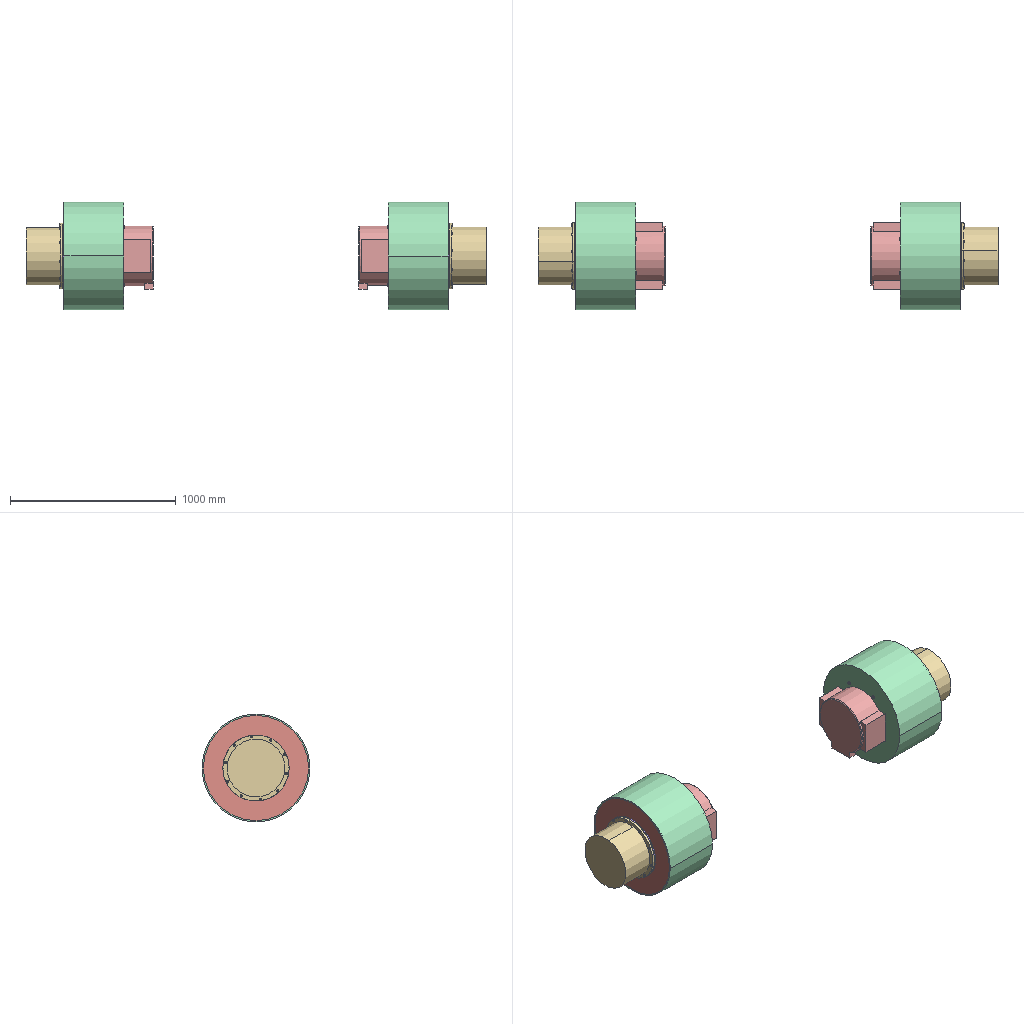Assembly | SolidWorks | 47 different items | 123 placed | box 2772 x 650 x 650 mm
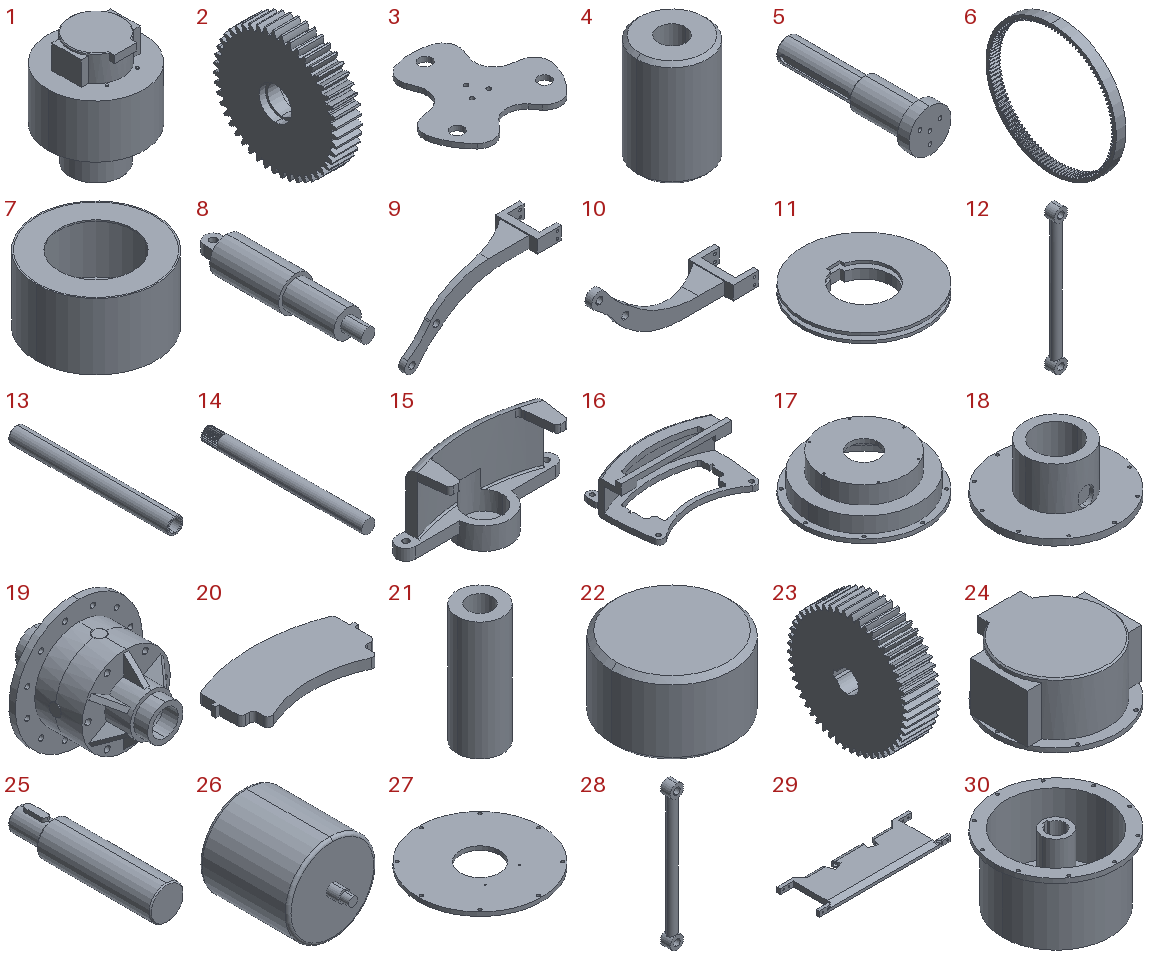Parts list (item | name | quantity | parent item | size | volume | features):
1 | (subassembly) | x2 | - | - | 73986218 mm3 | features CompositeCurve 5
2 | - | x6 | in 1 | 40 x 195.86 x 195.96 mm | 1021881 mm3 | features ICE 1, MBimport 1, MirrorPattern 1
3 | - | x2 | in 1 | 391.135 x 357.967 x 15 mm | 1196806 mm3 | features ICE 2, Extrusion 1, Fillet 1
4 | - | x6 | in 1 | 40 x 40 x 60 mm | 63591 mm3 | features Chamfer 1, Extrusion 1, HoleWzd 1
5 | - | x2 | in 1 | 110 x 370 x 110 mm | 1516861 mm3 | features HoleWzd 2, ICE 2, Chamfer 1, Fillet 1, Revolution 1
6 | - | x2 | in 1 | 40 x 530 x 530 mm | 927581 mm3 | features ICE 1, MBimport 1
7 | - | x2 | in 1 | 650 x 650 x 360 mm | 8402293 mm3 | features ICE 3, Cut 1, Extrusion 1
8 | - | x1 | - | 100 x 475 x 100 mm | 2480204 mm3 | features ICE 1, Revolution 1
9 | - | x1 | - | 920 x 260 x 385 mm | 5252996 mm3 | features ICE 3, Cut 1, Extrusion 1
10 | - | x1 | - | 920 x 260 x 385 mm | 5479591 mm3 | features ICE 3, Cut 1, Extrusion 1, MirrorSolid 1
11 | - | x2 | in 1 | 451 x 451 x 60 mm | 3289063 mm3 | features ICE 3, Extrusion 1, MirrorSolid 1
12 | - | x1 | - | 90 x 67.5 x 990 mm | 2949409 mm3 | features ICE 2, Extrusion 1, Scale 1
13 | - | x1 | - | 70 x 687.27 x 70 mm | 1240304 mm3 | features MBimport 1
14 | - | x1 | - | 51 x 611.661 x 51 mm | 1227372 mm3 | features ICE 1, MBimport 1
15 | - | x2 | in 1 | 215 x 70 x 107.5 mm | 333533 mm3 | features Fillet 5, ICE 5, Extrusion 1
16 | - | x2 | in 1 | 210 x 140.109 x 75 mm | 309603 mm3 | features ICE 5, Fillet 4, Cut 1, Extrusion 1, Shell 1
17 | - | x2 | in 1 | 630 x 630 x 190 mm | 10873138 mm3 | features ICE 5, Extrusion 1, HoleWzd 1
18 | - | x2 | in 1 | 400 x 400 x 160 mm | 4551688 mm3 | features ICE 2, Cut 1, Extrusion 1, Fillet 1
19 | - | x1 | - | 250 x 260.308 x 250 mm | 2320468 mm3 | features BaseBody 3
20 | - | x4 | in 1 | 175 x 84.844 x 12 mm | 137582 mm3 | features ICE 2, Extrusion 1, Fillet 1
21 | - | x4 | in 1 | 15 x 15 x 39 mm | 4932 mm3 | features Extrusion 1
22 | - | x2 | in 1 | 50 x 50 x 30 mm | 58293 mm3 | features Chamfer 1, Extrusion 1
23 | - | x2 | in 1 | 30 x 107.874 x 107.874 mm | 241879 mm3 | features ICE 1, MBimport 1
24 | - | x2 | in 1 | 430 x 430 x 200 mm | 23043977 mm3 | features ICE 4, Chamfer 1, Extrusion 1, MirrorPattern 1
25 | - | x2 | in 1 | 30 x 130 x 30 mm | 78732 mm3 | features Chamfer 1, Fillet 1, HoleWzd 1, ICE 1, Revolution 1
26 | - | x1 | - | 300 x 370 x 300 mm | 21237373 mm3 | features Fillet 1, Revolution 1
27 | - | x2 | in 1 | 630 x 630 x 20 mm | 5575887 mm3 | features Cut 1, Extrusion 1
28 | - | x1 | - | 120 x 90 x 1320 mm | 6991195 mm3 | features ICE 2, Extrusion 1, Scale 1
29 | - | x1 | - | 1500 x 480 x 60 mm | 30002400 mm3 | features Fillet 5, ICE 4, Chamfer 2, Cut 1, Extrusion 1, MirrorPattern 1
30 | - | x2 | in 1 | 400 x 400 x 220 mm | 6200986 mm3 | features ICE 4, Extrusion 1
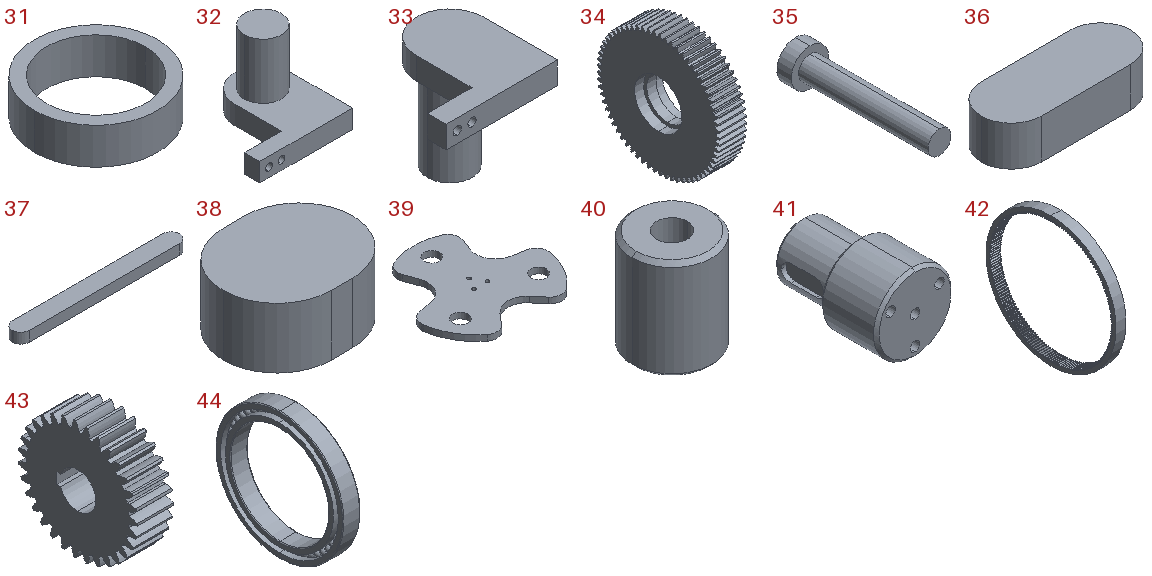31 | - | x2 | in 1 | 100 x 100 x 29.5 mm | 83409 mm3 | features Extrusion 1
32 | - | x1 | - | 150 x 145 x 120 mm | 660143 mm3 | features ICE 3, Extrusion 1
33 | - | x1 | - | 150 x 145 x 150 mm | 744966 mm3 | features ICE 3, Extrusion 1
34 | - | x6 | in 1 | 30 x 133.951 x 133.986 mm | 336105 mm3 | features ICE 2, MBimport 1, MirrorPattern 1
35 | - | x4 | in 1 | 13 x 50 x 13 mm | 2926 mm3 | features Revolution 1
36 | - | x2 | in 1 | 30 x 12 x 8 mm | 2633 mm3 | features Extrusion 1, Fillet 1
37 | - | x2 | in 1 | 180 x 18 x 11 mm | 34875 mm3 | features Extrusion 1, Fillet 1
38 | - | x2 | in 1 | 60 x 50 x 28 mm | 68978 mm3 | features Extrusion 1, Fillet 1
39 | - | x2 | in 1 | 327.043 x 300.67 x 15 mm | 824614 mm3 | features ICE 2, Extrusion 1, Fillet 1
40 | - | x6 | in 1 | 40 x 40 x 50 mm | 52911 mm3 | features Chamfer 1, Extrusion 1, HoleWzd 1
41 | - | x2 | in 1 | 55 x 80 x 55 mm | 132055 mm3 | features HoleWzd 2, Chamfer 1, Fillet 1, ICE 1, Revolution 1
42 | - | x2 | in 1 | 30 x 390 x 390 mm | 449494 mm3 | features ICE 1, MBimport 1, MoveFace 1
43 | - | x2 | in 1 | 40 x 131.774 x 131.932 mm | 421323 mm3 | features MBimport 1
44 | - | x24 | in 1 | 7 x 52 x 52 mm | 4483 mm3 | features MBimport 1
45 | hexagon head bolts-full thread gb | x1 | - | - | - | -
46 | tapered roller bearings gb | x1 | - | - | - | -
47 | Integral Axle Housing | x1 | - | - | - | -
Mates (type | each side: item.copy, entity, surface, feature):
In the top assembly
Coincident | 24.1 face plane Boss-Extrude3 | 24.2 face plane Boss-Extrude3
Concentric | 30.1 face cylinder Boss-Extrude1 | 24.2 face cylinder Boss-Extrude1
In subassembly 1
Coincident | 23.1 face plane Stage1 sun gear M2-T52.STEP | 1.1 plane
DistanceDim | 1.1 plane | 23.1 face cylinder Stage1 sun gear M2-T52.STEP | 2 times
Coincident | 23.1 face plane Stage1 sun gear M2-T52.STEP | 34.1 face plane Stage1 planet gear M2-T65.STEP
Coincident | 42.1 edge | 34.1 face plane Stage1 planet gear M2-T65.STEP
Concentric | 23.1 face cylinder Stage1 sun gear M2-T52.STEP | 42.1 face cylinder Boss-Extrude1
Concentric | 34.1 face cylinder Stage1 planet gear M2-T65.STEP | 40.1 face cylinder Boss-Extrude1 | 2 times
Concentric | 44.1 face cylinder 61808 bearing.STEP | 40.1 face cylinder Boss-Extrude1
Concentric | 44.1 face cylinder 61808 bearing.STEP | 44.2 face cylinder 61808 bearing.STEP
Coincident | 44.1 face plane 61808 bearing.STEP | 34.1 face plane Mirror1
Coincident | 34.1 face plane Cut-Extrude1 | 44.2 face plane 61808 bearing.STEP
Concentric | 42.1 face cylinder Boss-Extrude1 | 39.1 face cylinder Boss-Extrude1
Concentric | 40.1 face cylinder Boss-Extrude1 | 39.1 face cylinder Boss-Extrude1
Coincident | 40.1 face plane Boss-Extrude1 | 39.1 face plane Boss-Extrude1
Coincident | 40.1 face plane Boss-Extrude1 | 44.2 face plane 61808 bearing.STEP
Concentric | 44.3 face cylinder 61808 bearing.STEP | 44.4 face cylinder 61808 bearing.STEP
Concentric | 40.2 face cylinder Boss-Extrude1 | 44.4 face cylinder 61808 bearing.STEP
Concentric | 40.2 face cylinder Boss-Extrude1 | 34.2 face cylinder Stage1 planet gear M2-T65.STEP | 2 times
Coincident | 44.3 face plane 61808 bearing.STEP | 34.2 face plane Cut-Extrude1
Coincident | 34.2 face plane Mirror1 | 44.4 face plane 61808 bearing.STEP
Coincident | 44.3 face plane 61808 bearing.STEP | 40.2 face plane Boss-Extrude1
Concentric | 44.5 face cylinder 61808 bearing.STEP | 44.6 face cylinder 61808 bearing.STEP
Concentric | 40.3 face cylinder Boss-Extrude1 | 44.6 face cylinder 61808 bearing.STEP
Concentric | 40.3 face cylinder Boss-Extrude1 | 34.3 face cylinder Stage1 planet gear M2-T65.STEP | 2 times
Coincident | 44.5 face plane 61808 bearing.STEP | 34.3 face plane Cut-Extrude1
Coincident | 34.3 face plane Mirror1 | 44.6 face plane 61808 bearing.STEP
Coincident | 40.3 face plane Boss-Extrude1 | 44.5 face plane 61808 bearing.STEP
Coincident | 34.2 face plane Stage1 planet gear M2-T65.STEP | 34.3 face plane Stage1 planet gear M2-T65.STEP
Coincident | 39.1 face plane Boss-Extrude1 | 40.2 face plane Boss-Extrude1
Concentric | 39.1 face cylinder Boss-Extrude1 | 40.2 face cylinder M18 Tapped Hole1
Concentric | 39.1 face cylinder Boss-Extrude1 | 40.3 face cylinder M18 Tapped Hole1
Concentric | 39.1 face cylinder Boss-Extrude1 | 41.1 face cylinder Revolve1
Coincident | 39.1 face plane Boss-Extrude1 | 41.1 face plane Revolve1
Coincident | 43.1 face plane Stage2 sun gear M4-T31.STEP | 2.1 face plane Stage2 planet gear M4-T41.STEP
Coincident | 6.1 face plane Stage2 ring gear M4-T125.STEP | 43.1 face plane Stage2 sun gear M4-T31.STEP
Concentric | 6.1 face cylinder Boss-Extrude1 | 43.1 face cylinder Stage2 sun gear M4-T31.STEP
Concentric | 41.1 face cylinder Revolve1 | 43.1 face cylinder Stage2 sun gear M4-T31.STEP
Coincident | 41.1 face plane Revolve1 | 43.1 face plane Stage2 sun gear M4-T31.STEP
Coincident | 41.1 face plane Cut-Extrude1 | 36.1 face plane Boss-Extrude1
Concentric | 41.1 face cylinder Fillet1 | 36.1 face cylinder Fillet1
Parallel | 41.1 face plane Cut-Extrude1 | 36.1 face plane Boss-Extrude1
Coincident | 43.1 face plane Stage2 sun gear M4-T31.STEP | 36.1 face plane Boss-Extrude1
Concentric | 44.7 face cylinder 61808 bearing.STEP | 44.8 face cylinder 61808 bearing.STEP
Concentric | 2.1 face cylinder Mirror1 | 44.7 face cylinder 61808 bearing.STEP
Coincident | 2.1 face plane Cut-Extrude1 | 44.8 face plane 61808 bearing.STEP
Coincident | 2.1 face plane Mirror1 | 44.7 face plane 61808 bearing.STEP
Concentric | 24.3 face cylinder Boss-Extrude1 | 42.1 face cylinder Boss-Extrude1
Concentric | 2.1 face cylinder Stage2 planet gear M4-T41.STEP | 4.1 face cylinder Boss-Extrude1
Coincident | 44.8 face plane 61808 bearing.STEP | 4.1 face plane Boss-Extrude1
Concentric | 6.1 face cylinder Boss-Extrude1 | 3.1 face cylinder Boss-Extrude1
Concentric | 3.1 face cylinder Boss-Extrude1 | 4.1 face cylinder Boss-Extrude1
Coincident | 3.1 face plane Boss-Extrude1 | 4.1 face plane Boss-Extrude1
Coincident | 2.2 face plane Mirror1 | 44.9 face plane 61808 bearing.STEP
Concentric | 44.9 face cylinder 61808 bearing.STEP | 44.10 face cylinder 61808 bearing.STEP
Coincident | 2.2 face plane Cut-Extrude1 | 44.10 face plane 61808 bearing.STEP
Concentric | 2.2 face cylinder Mirror1 | 44.9 face cylinder 61808 bearing.STEP
Coincident | 44.10 face plane 61808 bearing.STEP | 4.2 face plane Boss-Extrude1
Concentric | 2.2 face cylinder Stage2 planet gear M4-T41.STEP | 4.2 face cylinder Boss-Extrude1
Coincident | 44.11 face plane 61808 bearing.STEP | 2.3 face plane Mirror1
Concentric | 44.11 face cylinder 61808 bearing.STEP | 44.12 face cylinder 61808 bearing.STEP
Coincident | 2.3 face plane Cut-Extrude1 | 44.12 face plane 61808 bearing.STEP
Concentric | 44.11 face cylinder 61808 bearing.STEP | 2.3 face cylinder Mirror1
Coincident | 44.12 face plane 61808 bearing.STEP | 4.3 face plane Boss-Extrude1
Concentric | 2.3 face cylinder Stage2 planet gear M4-T41.STEP | 4.3 face cylinder Boss-Extrude1
Coincident | 2.2 face plane Stage2 planet gear M4-T41.STEP | 2.3 face plane Stage2 planet gear M4-T41.STEP
Concentric | 3.1 face cylinder Boss-Extrude1 | 4.2 face cylinder Boss-Extrude1
Concentric | 3.1 face cylinder Boss-Extrude1 | 4.3 face cylinder Boss-Extrude1
Coincident | 6.1 face plane Stage2 ring gear M4-T125.STEP | 2.2 face plane Stage2 planet gear M4-T41.STEP
Concentric | 24.3 face cylinder Boss-Extrude1 | 25.1 face cylinder Revolve1
Coincident | 24.3 face plane Cut-Extrude1 | 25.1 face plane Revolve1
Coincident | 42.1 face plane Stage1 ring gear M2-T182.STEP | 25.1 face plane Revolve1
Parallel | 23.1 face plane Stage1 sun gear M2-T52.STEP | 25.1 face plane Boss-Extrude1
Concentric | 39.1 face cylinder Cut-Extrude2 | 41.1 face cylinder M8 Tapped Hole1
Concentric | 3.1 face cylinder Boss-Extrude1 | 5.1 face cylinder Revolve1
Coincident | 3.1 face plane Boss-Extrude1 | 5.1 face plane Revolve1
Coincident | 5.1 face plane Cut-Extrude1 | 37.1 face plane Boss-Extrude1 | 2 times
Concentric | 5.1 face cylinder Fillet1 | 37.1 face cylinder Fillet1
Concentric | 3.1 edge | 5.1 face cylinder M12 Tapped Hole1
Concentric | 5.1 face cylinder Revolve1 | 30.2 face cylinder Boss-Extrude1
Coincident | 5.1 face plane Revolve1 | 30.2 face plane Boss-Extrude1
Coincident | 5.1 face plane Cut-Extrude1 | 30.2 face plane Cut-Extrude2
Coincident | 30.2 face plane Boss-Extrude1 | 18.1 face plane Boss-Extrude1
Concentric | 30.2 face cylinder Boss-Extrude2 | 18.1 face cylinder Boss-Extrude1 | 2 times
Concentric | 42.1 face cylinder Boss-Extrude1 | 17.1 face cylinder Boss-Extrude1
Coincident | 24.3 face plane Boss-Extrude1 | 17.1 face plane Boss-Extrude1
Parallel | 17.1 plane | 1.1 plane
Concentric | 5.1 face cylinder Revolve1 | 31.1 face cylinder Boss-Extrude1
Concentric | 30.2 face cylinder Boss-Extrude1 | 27.1 face cylinder Boss-Extrude1
Coincident | 17.1 face plane Boss-Extrude2 | 27.1 face plane Boss-Extrude1
Concentric | 17.1 face cylinder Boss-Extrude4 | 27.1 face cylinder Boss-Extrude1
Concentric | 18.1 face cylinder Boss-Extrude2 | 11.1 face cylinder Mirror1
DistanceDim | 11.1 face plane Mirror1 | 18.1 face plane Boss-Extrude1
Coincident | 18.1 face plane Cut-Extrude2 | 11.1 face plane Cut-Extrude1
Coincident | 18.1 face plane Cut-Extrude2 | 38.1 face plane Boss-Extrude1
Parallel | 18.1 face plane Cut-Extrude2 | 38.1 face plane Boss-Extrude1
Concentric | 20.1 face cylinder Boss-Extrude1 | 20.2 face cylinder Boss-Extrude1
Coincident | 20.1 face plane Boss-Extrude1 | 20.2 face plane Boss-Extrude1
Concentric | 20.1 face cylinder Boss-Extrude1 | 15.1 face cylinder Boss-Extrude1
Concentric | 15.1 face cylinder Boss-Extrude3 | 22.1 face cylinder Boss-Extrude1
Coincident | 20.2 face plane Boss-Extrude1 | 22.1 face plane Boss-Extrude1
Concentric | 11.1 face cylinder Mirror1 | 20.1 face cylinder Boss-Extrude1
Parallel | 20.1 plane | 1.1 plane
Parallel | 15.1 plane | 1.1 plane
DistanceDim | 18.1 face plane Boss-Extrude1 | 15.1 face plane Boss-Extrude1
Concentric | 18.1 face cylinder Fillet1 | 38.1 face cylinder Fillet1
Parallel | 24.3 plane | 1.1 plane
Concentric | 15.1 face cylinder Boss-Extrude1 | 16.1 face cylinder Boss-Extrude1
Parallel | 16.1 plane | 1.1 plane
Coincident | 15.1 face plane Boss-Extrude2 | 16.1 face plane Boss-Extrude1
Coincident | 20.1 face plane Boss-Extrude1 | 16.1 face plane Boss-Extrude1
Coincident | 35.1 edge | 35.2 face plane Revolve1
Coincident | 16.1 face plane Boss-Extrude3 | 35.1 face plane Revolve1
Concentric | 16.1 face cylinder Boss-Extrude3 | 35.2 face cylinder Revolve1
Concentric | 16.1 face cylinder Boss-Extrude3 | 35.1 face cylinder Revolve1
Coincident | 21.1 face plane Boss-Extrude1 | 21.2 face plane Boss-Extrude1
Coincident | 16.1 face plane Boss-Extrude1 | 21.2 face plane Boss-Extrude1
Concentric | 16.1 edge | 21.2 face cylinder Boss-Extrude1
Concentric | 16.1 face cylinder Fillet2 | 21.1 face cylinder Boss-Extrude1
Concentric | 24.3 face cylinder Boss-Extrude1 | 7.1 face cylinder Boss-Extrude1
Coincident | 24.3 face plane Boss-Extrude4 | 7.1 face plane Cut-Extrude2
Parallel | 7.1 plane | 1.1 plane